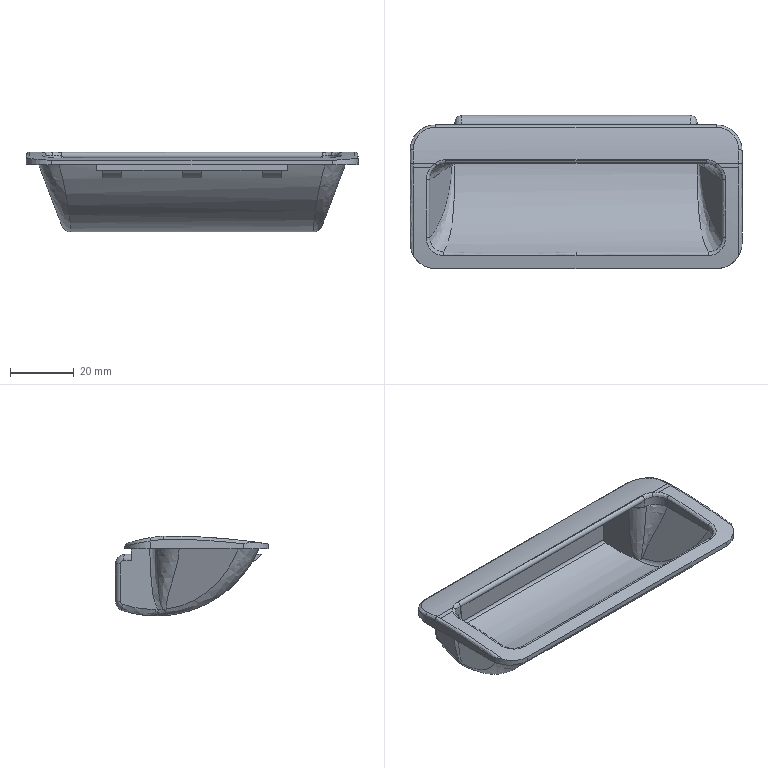Part | STEP file | 1 solid | 112 faces | box 104 x 48 x 25.005 mm | volume 18990 mm3 | spline 49 | plane 34 | cylinder 29 | commonest cylinder face diameters 2 x6 4 x4 16 x4 12 x3 400 x3 6 x2